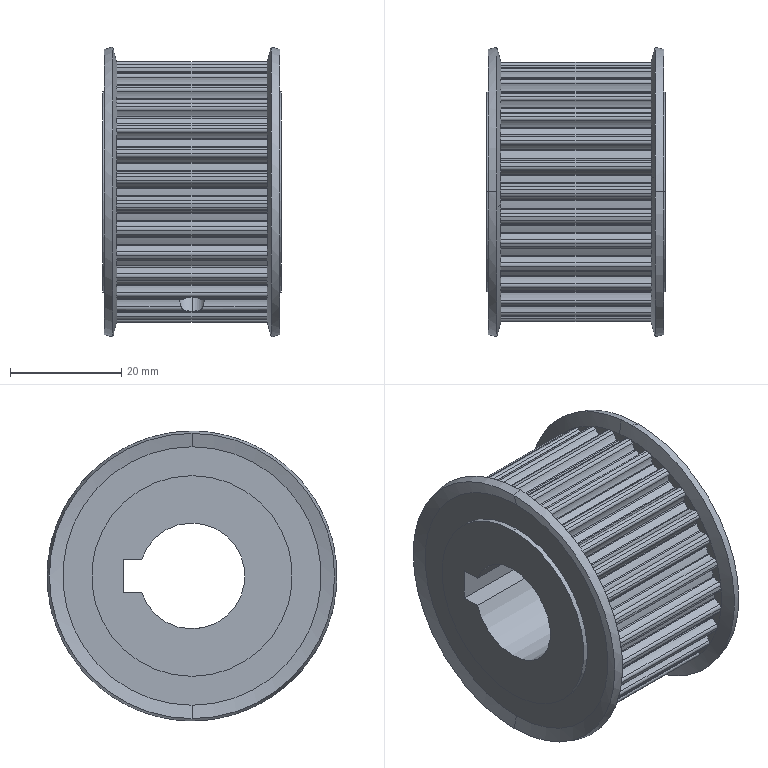Part | STEP file | timing pulley C-HTPA30S5M250-A-N19 | 1 solid | 342 faces | box 32 x 52 x 52 mm | volume 41096 mm3 | cylinder 263 | plane 67 | cone 12 | commonest cylinder face diameters 0.5 x64 1.1 x64 6.55 x64 43.25 x32 46.79 x30 4.917 x4